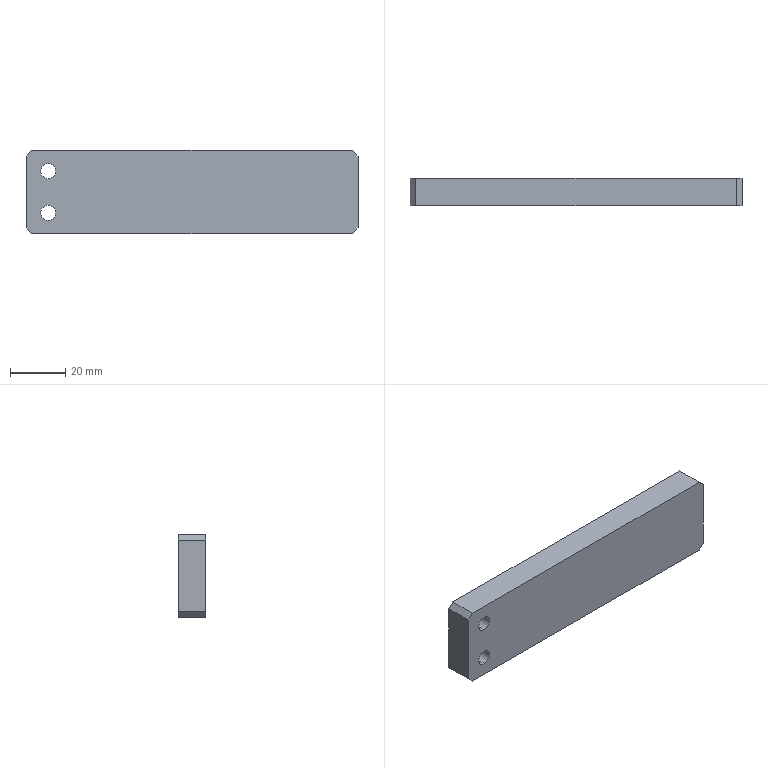Part | SolidWorks | features HoleWzd 2, BreakCorner 1, FlatPattern 1, SMBaseFlange 1, SheetMetal 1 | 1 solid | 22 faces | box 120 x 10 x 30 mm | volume 35369 mm3 | plane 10 | cylinder 8 | cone 4 | commonest cylinder face diameters 2.5 x4 5.5 x4
STEP:
#1=CARTESIAN_POINT('',(43.5,-7.5,-16.25));
#2=VERTEX_POINT('',#1);
#3=CARTESIAN_POINT('',(43.5,-7.5,-13.75));
#4=VERTEX_POINT('',#3);
#5=CARTESIAN_POINT('',(43.5,-7.5,-15.));
#6=DIRECTION('',(0.,1.,0.));
#7=DIRECTION('',(0.,0.,1.));
#8=AXIS2_PLACEMENT_3D('',#5,#6,#7);
#9=CIRCLE('',#8,1.25);
#10=EDGE_CURVE('',#2,#4,#9,.T.);
#11=ORIENTED_EDGE('',*,*,#10,.F.);
#12=CARTESIAN_POINT('',(43.5,0.,-16.25));
#13=VERTEX_POINT('',#12);
#14=CARTESIAN_POINT('',(43.5,0.,-16.25));
#15=DIRECTION('',(0.,1.,0.));
#16=VECTOR('',#15,1000.);
#17=LINE('',#14,#16);
#18=EDGE_CURVE('',#2,#13,#17,.T.);
#19=ORIENTED_EDGE('',*,*,#18,.T.);
#20=CARTESIAN_POINT('',(43.5,0.,-13.75));
#21=VERTEX_POINT('',#20);
#22=CARTESIAN_POINT('',(43.5,0.,-15.));
#23=DIRECTION('',(0.,1.,0.));
#24=DIRECTION('',(0.,0.,1.));
#25=AXIS2_PLACEMENT_3D('',#22,#23,#24);
#26=CIRCLE('',#25,1.25);
#27=EDGE_CURVE('',#13,#21,#26,.T.);
#28=ORIENTED_EDGE('',*,*,#27,.T.);
#29=CARTESIAN_POINT('',(43.5,0.,-13.75));
#30=DIRECTION('',(0.,1.,0.));
#31=VECTOR('',#30,1000.);
#32=LINE('',#29,#31);
#33=EDGE_CURVE('',#4,#21,#32,.T.);
#34=ORIENTED_EDGE('',*,*,#33,.F.);
#35=EDGE_LOOP('',(#11,#19,#28,#34));
#36=FACE_OUTER_BOUND('',#35,.T.);
#37=CARTESIAN_POINT('',(43.5,0.,-15.));
#38=DIRECTION('',(0.,1.,0.));
#39=DIRECTION('',(0.,0.,1.));
#40=AXIS2_PLACEMENT_3D('',#37,#38,#39);
#41=CYLINDRICAL_SURFACE('',#40,1.25);
#42=ADVANCED_FACE('',(#36),#41,.F.);
#43=CARTESIAN_POINT('',(43.5,-8.251,-15.));
#44=VERTEX_POINT('',#43);
#45=CARTESIAN_POINT('',(43.5,-7.5,-13.75));
#46=DIRECTION('',(0.,0.515,0.8572));
#47=VECTOR('',#46,1000.);
#48=LINE('',#45,#47);
#49=EDGE_CURVE('',#44,#4,#48,.T.);
#50=ORIENTED_EDGE('',*,*,#49,.F.);
#51=CARTESIAN_POINT('',(43.5,-7.5,-16.25));
#52=DIRECTION('',(0.,0.515,-0.8572));
#53=VECTOR('',#52,1000.);
#54=LINE('',#51,#53);
#55=EDGE_CURVE('',#44,#2,#54,.T.);
#56=ORIENTED_EDGE('',*,*,#55,.T.);
#57=ORIENTED_EDGE('',*,*,#10,.T.);
#58=EDGE_LOOP('',(#50,#56,#57));
#59=FACE_OUTER_BOUND('',#58,.T.);
#60=CARTESIAN_POINT('',(43.5,-7.5,-15.));
#61=DIRECTION('',(0.,1.,0.));
#62=DIRECTION('',(0.,0.,1.));
#63=AXIS2_PLACEMENT_3D('',#60,#61,#62);
#64=CONICAL_SURFACE('',#63,1.25,1.03);
#65=ADVANCED_FACE('',(#59),#64,.F.);
#66=CARTESIAN_POINT('',(93.5,-7.5,-16.25));
#67=VERTEX_POINT('',#66);
#68=CARTESIAN_POINT('',(93.5,-7.5,-13.75));
#69=VERTEX_POINT('',#68);
#70=CARTESIAN_POINT('',(93.5,-7.5,-15.));
#71=DIRECTION('',(0.,1.,0.));
#72=DIRECTION('',(0.,0.,1.));
#73=AXIS2_PLACEMENT_3D('',#70,#71,#72);
#74=CIRCLE('',#73,1.25);
#75=EDGE_CURVE('',#67,#69,#74,.T.);
#76=ORIENTED_EDGE('',*,*,#75,.F.);
#77=CARTESIAN_POINT('',(93.5,0.,-16.25));
#78=VERTEX_POINT('',#77);
#79=CARTESIAN_POINT('',(93.5,0.,-16.25));
#80=DIRECTION('',(0.,1.,0.));
#81=VECTOR('',#80,1000.);
#82=LINE('',#79,#81);
#83=EDGE_CURVE('',#67,#78,#82,.T.);
#84=ORIENTED_EDGE('',*,*,#83,.T.);
#85=CARTESIAN_POINT('',(93.5,0.,-13.75));
#86=VERTEX_POINT('',#85);
#87=CARTESIAN_POINT('',(93.5,0.,-15.));
#88=DIRECTION('',(0.,1.,0.));
#89=DIRECTION('',(0.,0.,1.));
#90=AXIS2_PLACEMENT_3D('',#87,#88,#89);
#91=CIRCLE('',#90,1.25);
#92=EDGE_CURVE('',#78,#86,#91,.T.);
#93=ORIENTED_EDGE('',*,*,#92,.T.);
#94=CARTESIAN_POINT('',(93.5,0.,-13.75));
#95=DIRECTION('',(0.,1.,0.));
#96=VECTOR('',#95,1000.);
#97=LINE('',#94,#96);
#98=EDGE_CURVE('',#69,#86,#97,.T.);
#99=ORIENTED_EDGE('',*,*,#98,.F.);
#100=EDGE_LOOP('',(#76,#84,#93,#99));
#101=FACE_OUTER_BOUND('',#100,.T.);
#102=CARTESIAN_POINT('',(93.5,0.,-15.));
#103=DIRECTION('',(0.,1.,0.));
#104=DIRECTION('',(0.,0.,1.));
#105=AXIS2_PLACEMENT_3D('',#102,#103,#104);
#106=CYLINDRICAL_SURFACE('',#105,1.25);
#107=ADVANCED_FACE('',(#101),#106,.F.);
#108=CARTESIAN_POINT('',(93.5,-8.251,-15.));
#109=VERTEX_POINT('',#108);
#110=CARTESIAN_POINT('',(93.5,-7.5,-13.75));
#111=DIRECTION('',(0.,0.515,0.8572));
#112=VECTOR('',#111,1000.);
#113=LINE('',#110,#112);
#114=EDGE_CURVE('',#109,#69,#113,.T.);
#115=ORIENTED_EDGE('',*,*,#114,.F.);
#116=CARTESIAN_POINT('',(93.5,-7.5,-16.25));
#117=DIRECTION('',(0.,0.515,-0.8572));
#118=VECTOR('',#117,1000.);
#119=LINE('',#116,#118);
#120=EDGE_CURVE('',#109,#67,#119,.T.);
#121=ORIENTED_EDGE('',*,*,#120,.T.);
#122=ORIENTED_EDGE('',*,*,#75,.T.);
#123=EDGE_LOOP('',(#115,#121,#122));
#124=FACE_OUTER_BOUND('',#123,.T.);
#125=CARTESIAN_POINT('',(93.5,-7.5,-15.));
#126=DIRECTION('',(0.,1.,0.));
#127=DIRECTION('',(0.,0.,1.));
#128=AXIS2_PLACEMENT_3D('',#125,#126,#127);
#129=CONICAL_SURFACE('',#128,1.25,1.03);
#130=ADVANCED_FACE('',(#124),#129,.F.);
#131=CARTESIAN_POINT('',(8.,0.,-19.75));
#132=VERTEX_POINT('',#131);
#133=CARTESIAN_POINT('',(8.,0.,-25.25));
#134=VERTEX_POINT('',#133);
#135=CARTESIAN_POINT('',(8.,0.,-22.5));
#136=DIRECTION('',(0.,-1.,0.));
#137=DIRECTION('',(0.,0.,-1.));
#138=AXIS2_PLACEMENT_3D('',#135,#136,#137);
#139=CIRCLE('',#138,2.75);
#140=EDGE_CURVE('',#132,#134,#139,.T.);
#141=ORIENTED_EDGE('',*,*,#140,.F.);
#142=CARTESIAN_POINT('',(8.,-10.,-19.75));
#143=VERTEX_POINT('',#142);
#144=CARTESIAN_POINT('',(8.,-10.,-19.75));
#145=DIRECTION('',(0.,-1.,0.));
#146=VECTOR('',#145,1000.);
#147=LINE('',#144,#146);
#148=EDGE_CURVE('',#132,#143,#147,.T.);
#149=ORIENTED_EDGE('',*,*,#148,.T.);
#150=CARTESIAN_POINT('',(8.,-10.,-25.25));
#151=VERTEX_POINT('',#150);
#152=CARTESIAN_POINT('',(8.,-10.,-22.5));
#153=DIRECTION('',(0.,-1.,0.));
#154=DIRECTION('',(0.,0.,-1.));
#155=AXIS2_PLACEMENT_3D('',#152,#153,#154);
#156=CIRCLE('',#155,2.75);
#157=EDGE_CURVE('',#143,#151,#156,.T.);
#158=ORIENTED_EDGE('',*,*,#157,.T.);
#159=CARTESIAN_POINT('',(8.,-10.,-25.25));
#160=DIRECTION('',(0.,-1.,0.));
#161=VECTOR('',#160,1000.);
#162=LINE('',#159,#161);
#163=EDGE_CURVE('',#134,#151,#162,.T.);
#164=ORIENTED_EDGE('',*,*,#163,.F.);
#165=EDGE_LOOP('',(#141,#149,#158,#164));
#166=FACE_OUTER_BOUND('',#165,.T.);
#167=CARTESIAN_POINT('',(8.,-10.,-22.5));
#168=DIRECTION('',(0.,-1.,0.));
#169=DIRECTION('',(0.,0.,-1.));
#170=AXIS2_PLACEMENT_3D('',#167,#168,#169);
#171=CYLINDRICAL_SURFACE('',#170,2.75);
#172=ADVANCED_FACE('',(#166),#171,.F.);
#173=CARTESIAN_POINT('',(8.,0.,-4.75));
#174=VERTEX_POINT('',#173);
#175=CARTESIAN_POINT('',(8.,0.,-10.25));
#176=VERTEX_POINT('',#175);
#177=CARTESIAN_POINT('',(8.,0.,-7.5));
#178=DIRECTION('',(0.,-1.,0.));
#179=DIRECTION('',(0.,0.,-1.));
#180=AXIS2_PLACEMENT_3D('',#177,#178,#179);
#181=CIRCLE('',#180,2.75);
#182=EDGE_CURVE('',#174,#176,#181,.T.);
#183=ORIENTED_EDGE('',*,*,#182,.F.);
#184=CARTESIAN_POINT('',(8.,-10.,-4.75));
#185=VERTEX_POINT('',#184);
#186=CARTESIAN_POINT('',(8.,-10.,-4.75));
#187=DIRECTION('',(0.,-1.,0.));
#188=VECTOR('',#187,1000.);
#189=LINE('',#186,#188);
#190=EDGE_CURVE('',#174,#185,#189,.T.);
#191=ORIENTED_EDGE('',*,*,#190,.T.);
#192=CARTESIAN_POINT('',(8.,-10.,-10.25));
#193=VERTEX_POINT('',#192);
#194=CARTESIAN_POINT('',(8.,-10.,-7.5));
#195=DIRECTION('',(0.,-1.,0.));
#196=DIRECTION('',(0.,0.,-1.));
#197=AXIS2_PLACEMENT_3D('',#194,#195,#196);
#198=CIRCLE('',#197,2.75);
#199=EDGE_CURVE('',#185,#193,#198,.T.);
#200=ORIENTED_EDGE('',*,*,#199,.T.);
#201=CARTESIAN_POINT('',(8.,-10.,-10.25));
#202=DIRECTION('',(0.,-1.,0.));
#203=VECTOR('',#202,1000.);
#204=LINE('',#201,#203);
#205=EDGE_CURVE('',#176,#193,#204,.T.);
#206=ORIENTED_EDGE('',*,*,#205,.F.);
#207=EDGE_LOOP('',(#183,#191,#200,#206));
#208=FACE_OUTER_BOUND('',#207,.T.);
#209=CARTESIAN_POINT('',(8.,-10.,-7.5));
#210=DIRECTION('',(0.,-1.,0.));
#211=DIRECTION('',(0.,0.,-1.));
#212=AXIS2_PLACEMENT_3D('',#209,#210,#211);
#213=CYLINDRICAL_SURFACE('',#212,2.75);
#214=ADVANCED_FACE('',(#208),#213,.F.);
#215=CARTESIAN_POINT('',(0.,-10.,-28.));
#216=VERTEX_POINT('',#215);
#217=CARTESIAN_POINT('',(0.,-10.,-2.));
#218=VERTEX_POINT('',#217);
#219=CARTESIAN_POINT('',(0.,-10.,0.));
#220=DIRECTION('',(0.,0.,1.));
#221=VECTOR('',#220,1000.);
#222=LINE('',#219,#221);
#223=EDGE_CURVE('',#216,#218,#222,.T.);
#224=ORIENTED_EDGE('',*,*,#223,.T.);
#225=CARTESIAN_POINT('',(0.,0.,-2.));
#226=VERTEX_POINT('',#225);
#227=CARTESIAN_POINT('',(0.,-10.,-2.));
#228=DIRECTION('',(0.,1.,0.));
#229=VECTOR('',#228,1000.);
#230=LINE('',#227,#229);
#231=EDGE_CURVE('',#218,#226,#230,.T.);
#232=ORIENTED_EDGE('',*,*,#231,.T.);
#233=CARTESIAN_POINT('',(0.,0.,-28.));
#234=VERTEX_POINT('',#233);
#235=CARTESIAN_POINT('',(0.,0.,0.));
#236=DIRECTION('',(0.,0.,1.));
#237=VECTOR('',#236,1000.);
#238=LINE('',#235,#237);
#239=EDGE_CURVE('',#234,#226,#238,.T.);
#240=ORIENTED_EDGE('',*,*,#239,.F.);
#241=CARTESIAN_POINT('',(0.,-10.,-28.));
#242=DIRECTION('',(0.,-1.,0.));
#243=VECTOR('',#242,1000.);
#244=LINE('',#241,#243);
#245=EDGE_CURVE('',#234,#216,#244,.T.);
#246=ORIENTED_EDGE('',*,*,#245,.T.);
#247=EDGE_LOOP('',(#224,#232,#240,#246));
#248=FACE_OUTER_BOUND('',#247,.T.);
#249=CARTESIAN_POINT('',(0.,-10.,0.));
#250=DIRECTION('',(-1.,0.,0.));
#251=DIRECTION('',(0.,0.,1.));
#252=AXIS2_PLACEMENT_3D('',#249,#250,#251);
#253=PLANE('',#252);
#254=ADVANCED_FACE('',(#248),#253,.T.);
#255=CARTESIAN_POINT('',(118.,0.,-30.));
#256=VERTEX_POINT('',#255);
#257=CARTESIAN_POINT('',(2.,0.,-30.));
#258=VERTEX_POINT('',#257);
#259=CARTESIAN_POINT('',(0.,0.,-30.));
#260=DIRECTION('',(-1.,0.,0.));
#261=VECTOR('',#260,1000.);
#262=LINE('',#259,#261);
#263=EDGE_CURVE('',#256,#258,#262,.T.);
#264=ORIENTED_EDGE('',*,*,#263,.F.);
#265=CARTESIAN_POINT('',(118.,-10.,-30.));
#266=VERTEX_POINT('',#265);
#267=CARTESIAN_POINT('',(118.,-10.,-30.));
#268=DIRECTION('',(0.,-1.,0.));
#269=VECTOR('',#268,1000.);
#270=LINE('',#267,#269);
#271=EDGE_CURVE('',#256,#266,#270,.T.);
#272=ORIENTED_EDGE('',*,*,#271,.T.);
#273=CARTESIAN_POINT('',(2.,-10.,-30.));
#274=VERTEX_POINT('',#273);
#275=CARTESIAN_POINT('',(0.,-10.,-30.));
#276=DIRECTION('',(-1.,0.,0.));
#277=VECTOR('',#276,1000.);
#278=LINE('',#275,#277);
#279=EDGE_CURVE('',#266,#274,#278,.T.);
#280=ORIENTED_EDGE('',*,*,#279,.T.);
#281=CARTESIAN_POINT('',(2.,-10.,-30.));
#282=DIRECTION('',(0.,1.,0.));
#283=VECTOR('',#282,1000.);
#284=LINE('',#281,#283);
#285=EDGE_CURVE('',#274,#258,#284,.T.);
#286=ORIENTED_EDGE('',*,*,#285,.T.);
#287=EDGE_LOOP('',(#264,#272,#280,#286));
#288=FACE_OUTER_BOUND('',#287,.T.);
#289=CARTESIAN_POINT('',(0.,-10.,-30.));
#290=DIRECTION('',(0.,0.,-1.));
#291=DIRECTION('',(-1.,0.,0.));
#292=AXIS2_PLACEMENT_3D('',#289,#290,#291);
#293=PLANE('',#292);
#294=ADVANCED_FACE('',(#288),#293,.T.);
#295=CARTESIAN_POINT('',(120.,0.,-2.));
#296=VERTEX_POINT('',#295);
#297=CARTESIAN_POINT('',(120.,0.,-28.));
#298=VERTEX_POINT('',#297);
#299=CARTESIAN_POINT('',(120.,0.,0.));
#300=DIRECTION('',(0.,0.,-1.));
#301=VECTOR('',#300,1000.);
#302=LINE('',#299,#301);
#303=EDGE_CURVE('',#296,#298,#302,.T.);
#304=ORIENTED_EDGE('',*,*,#303,.F.);
#305=CARTESIAN_POINT('',(120.,-10.,-2.));
#306=VERTEX_POINT('',#305);
#307=CARTESIAN_POINT('',(120.,-10.,-2.));
#308=DIRECTION('',(0.,-1.,0.));
#309=VECTOR('',#308,1000.);
#310=LINE('',#307,#309);
#311=EDGE_CURVE('',#296,#306,#310,.T.);
#312=ORIENTED_EDGE('',*,*,#311,.T.);
#313=CARTESIAN_POINT('',(120.,-10.,-28.));
#314=VERTEX_POINT('',#313);
#315=CARTESIAN_POINT('',(120.,-10.,0.));
#316=DIRECTION('',(0.,0.,-1.));
#317=VECTOR('',#316,1000.);
#318=LINE('',#315,#317);
#319=EDGE_CURVE('',#306,#314,#318,.T.);
#320=ORIENTED_EDGE('',*,*,#319,.T.);
#321=CARTESIAN_POINT('',(120.,-10.,-28.));
#322=DIRECTION('',(0.,1.,0.));
#323=VECTOR('',#322,1000.);
#324=LINE('',#321,#323);
#325=EDGE_CURVE('',#314,#298,#324,.T.);
#326=ORIENTED_EDGE('',*,*,#325,.T.);
#327=EDGE_LOOP('',(#304,#312,#320,#326));
#328=FACE_OUTER_BOUND('',#327,.T.);
#329=CARTESIAN_POINT('',(120.,-10.,0.));
#330=DIRECTION('',(1.,0.,0.));
#331=DIRECTION('',(0.,0.,-1.));
#332=AXIS2_PLACEMENT_3D('',#329,#330,#331);
#333=PLANE('',#332);
#334=ADVANCED_FACE('',(#328),#333,.T.);
#335=CARTESIAN_POINT('',(2.,0.,0.));
#336=VERTEX_POINT('',#335);
#337=CARTESIAN_POINT('',(118.,0.,0.));
#338=VERTEX_POINT('',#337);
#339=CARTESIAN_POINT('',(0.,0.,0.));
#340=DIRECTION('',(1.,0.,0.));
#341=VECTOR('',#340,1000.);
#342=LINE('',#339,#341);
#343=EDGE_CURVE('',#336,#338,#342,.T.);
#344=ORIENTED_EDGE('',*,*,#343,.F.);
#345=CARTESIAN_POINT('',(2.,-10.,0.));
#346=VERTEX_POINT('',#345);
#347=CARTESIAN_POINT('',(2.,-10.,0.));
#348=DIRECTION('',(0.,-1.,0.));
#349=VECTOR('',#348,1000.);
#350=LINE('',#347,#349);
#351=EDGE_CURVE('',#336,#346,#350,.T.);
#352=ORIENTED_EDGE('',*,*,#351,.T.);
#353=CARTESIAN_POINT('',(118.,-10.,0.));
#354=VERTEX_POINT('',#353);
#355=CARTESIAN_POINT('',(0.,-10.,0.));
#356=DIRECTION('',(1.,0.,0.));
#357=VECTOR('',#356,1000.);
#358=LINE('',#355,#357);
#359=EDGE_CURVE('',#346,#354,#358,.T.);
#360=ORIENTED_EDGE('',*,*,#359,.T.);
#361=CARTESIAN_POINT('',(118.,-10.,0.));
#362=DIRECTION('',(0.,1.,0.));
#363=VECTOR('',#362,1000.);
#364=LINE('',#361,#363);
#365=EDGE_CURVE('',#354,#338,#364,.T.);
#366=ORIENTED_EDGE('',*,*,#365,.T.);
#367=EDGE_LOOP('',(#344,#352,#360,#366));
#368=FACE_OUTER_BOUND('',#367,.T.);
#369=CARTESIAN_POINT('',(0.,-10.,0.));
#370=DIRECTION('',(0.,0.,1.));
#371=DIRECTION('',(1.,0.,0.));
#372=AXIS2_PLACEMENT_3D('',#369,#370,#371);
#373=PLANE('',#372);
#374=ADVANCED_FACE('',(#368),#373,.T.);
#375=CARTESIAN_POINT('',(8.,-10.,-22.5));
#376=DIRECTION('',(0.,-1.,0.));
#377=DIRECTION('',(0.,0.,-1.));
#378=AXIS2_PLACEMENT_3D('',#375,#376,#377);
#379=CIRCLE('',#378,2.75);
#380=EDGE_CURVE('',#151,#143,#379,.T.);
#381=ORIENTED_EDGE('',*,*,#380,.F.);
#382=ORIENTED_EDGE('',*,*,#157,.F.);
#383=EDGE_LOOP('',(#381,#382));
#384=FACE_BOUND('',#383,.T.);
#385=CARTESIAN_POINT('',(8.,-10.,-7.5));
#386=DIRECTION('',(0.,-1.,0.));
#387=DIRECTION('',(0.,0.,-1.));
#388=AXIS2_PLACEMENT_3D('',#385,#386,#387);
#389=CIRCLE('',#388,2.75);
#390=EDGE_CURVE('',#193,#185,#389,.T.);
#391=ORIENTED_EDGE('',*,*,#390,.F.);
#392=ORIENTED_EDGE('',*,*,#199,.F.);
#393=EDGE_LOOP('',(#391,#392));
#394=FACE_BOUND('',#393,.T.);
#395=ORIENTED_EDGE('',*,*,#359,.F.);
#396=CARTESIAN_POINT('',(1.,-10.,-1.));
#397=DIRECTION('',(-0.7071,0.,-0.7071));
#398=VECTOR('',#397,1000.);
#399=LINE('',#396,#398);
#400=EDGE_CURVE('',#346,#218,#399,.T.);
#401=ORIENTED_EDGE('',*,*,#400,.T.);
#402=ORIENTED_EDGE('',*,*,#223,.F.);
#403=CARTESIAN_POINT('',(-14.,-10.,-14.));
#404=DIRECTION('',(0.7071,0.,-0.7071));
#405=VECTOR('',#404,1000.);
#406=LINE('',#403,#405);
#407=EDGE_CURVE('',#216,#274,#406,.T.);
#408=ORIENTED_EDGE('',*,*,#407,.T.);
#409=ORIENTED_EDGE('',*,*,#279,.F.);
#410=CARTESIAN_POINT('',(74.,-10.,-74.));
#411=DIRECTION('',(0.7071,0.,0.7071));
#412=VECTOR('',#411,1000.);
#413=LINE('',#410,#412);
#414=EDGE_CURVE('',#266,#314,#413,.T.);
#415=ORIENTED_EDGE('',*,*,#414,.T.);
#416=ORIENTED_EDGE('',*,*,#319,.F.);
#417=CARTESIAN_POINT('',(59.,-10.,59.));
#418=DIRECTION('',(-0.7071,0.,0.7071));
#419=VECTOR('',#418,1000.);
#420=LINE('',#417,#419);
#421=EDGE_CURVE('',#306,#354,#420,.T.);
#422=ORIENTED_EDGE('',*,*,#421,.T.);
#423=EDGE_LOOP('',(#395,#401,#402,#408,#409,#415,#416,#422));
#424=FACE_OUTER_BOUND('',#423,.T.);
#425=CARTESIAN_POINT('',(0.,-10.,0.));
#426=DIRECTION('',(0.,-1.,0.));
#427=DIRECTION('',(0.,0.,-1.));
#428=AXIS2_PLACEMENT_3D('',#425,#426,#427);
#429=PLANE('',#428);
#430=ADVANCED_FACE('',(#384,#394,#424),#429,.T.);
#431=CARTESIAN_POINT('',(43.5,0.,-15.));
#432=DIRECTION('',(0.,1.,0.));
#433=DIRECTION('',(0.,0.,1.));
#434=AXIS2_PLACEMENT_3D('',#431,#432,#433);
#435=CIRCLE('',#434,1.25);
#436=EDGE_CURVE('',#21,#13,#435,.T.);
#437=ORIENTED_EDGE('',*,*,#436,.F.);
#438=ORIENTED_EDGE('',*,*,#27,.F.);
#439=EDGE_LOOP('',(#437,#438));
#440=FACE_BOUND('',#439,.T.);
#441=CARTESIAN_POINT('',(93.5,0.,-15.));
#442=DIRECTION('',(0.,1.,0.));
#443=DIRECTION('',(0.,0.,1.));
#444=AXIS2_PLACEMENT_3D('',#441,#442,#443);
#445=CIRCLE('',#444,1.25);
#446=EDGE_CURVE('',#86,#78,#445,.T.);
#447=ORIENTED_EDGE('',*,*,#446,.F.);
#448=ORIENTED_EDGE('',*,*,#92,.F.);
#449=EDGE_LOOP('',(#447,#448));
#450=FACE_BOUND('',#449,.T.);
#451=CARTESIAN_POINT('',(8.,0.,-22.5));
#452=DIRECTION('',(0.,-1.,0.));
#453=DIRECTION('',(0.,0.,-1.));
#454=AXIS2_PLACEMENT_3D('',#451,#452,#453);
#455=CIRCLE('',#454,2.75);
#456=EDGE_CURVE('',#134,#132,#455,.T.);
#457=ORIENTED_EDGE('',*,*,#456,.T.);
#458=ORIENTED_EDGE('',*,*,#140,.T.);
#459=EDGE_LOOP('',(#457,#458));
#460=FACE_BOUND('',#459,.T.);
#461=CARTESIAN_POINT('',(8.,0.,-7.5));
#462=DIRECTION('',(0.,-1.,0.));
#463=DIRECTION('',(0.,0.,-1.));
#464=AXIS2_PLACEMENT_3D('',#461,#462,#463);
#465=CIRCLE('',#464,2.75);
#466=EDGE_CURVE('',#176,#174,#465,.T.);
#467=ORIENTED_EDGE('',*,*,#466,.T.);
#468=ORIENTED_EDGE('',*,*,#182,.T.);
#469=EDGE_LOOP('',(#467,#468));
#470=FACE_BOUND('',#469,.T.);
#471=ORIENTED_EDGE('',*,*,#239,.T.);
#472=CARTESIAN_POINT('',(0.,0.,-2.));
#473=DIRECTION('',(0.7071,0.,0.7071));
#474=VECTOR('',#473,1000.);
#475=LINE('',#472,#474);
#476=EDGE_CURVE('',#226,#336,#475,.T.);
#477=ORIENTED_EDGE('',*,*,#476,.T.);
#478=ORIENTED_EDGE('',*,*,#343,.T.);
#479=CARTESIAN_POINT('',(118.,0.,0.));
#480=DIRECTION('',(0.7071,0.,-0.7071));
#481=VECTOR('',#480,1000.);
#482=LINE('',#479,#481);
#483=EDGE_CURVE('',#338,#296,#482,.T.);
#484=ORIENTED_EDGE('',*,*,#483,.T.);
#485=ORIENTED_EDGE('',*,*,#303,.T.);
#486=CARTESIAN_POINT('',(120.,0.,-28.));
#487=DIRECTION('',(-0.7071,0.,-0.7071));
#488=VECTOR('',#487,1000.);
#489=LINE('',#486,#488);
#490=EDGE_CURVE('',#298,#256,#489,.T.);
#491=ORIENTED_EDGE('',*,*,#490,.T.);
#492=ORIENTED_EDGE('',*,*,#263,.T.);
#493=CARTESIAN_POINT('',(2.,0.,-30.));
#494=DIRECTION('',(-0.7071,0.,0.7071));
#495=VECTOR('',#494,1000.);
#496=LINE('',#493,#495);
#497=EDGE_CURVE('',#258,#234,#496,.T.);
#498=ORIENTED_EDGE('',*,*,#497,.T.);
#499=EDGE_LOOP('',(#471,#477,#478,#484,#485,#491,#492,#498));
#500=FACE_OUTER_BOUND('',#499,.T.);
#501=CARTESIAN_POINT('',(0.,0.,0.));
#502=DIRECTION('',(0.,-1.,0.));
#503=DIRECTION('',(0.,0.,-1.));
#504=AXIS2_PLACEMENT_3D('',#501,#502,#503);
#505=PLANE('',#504);
#506=ADVANCED_FACE('',(#440,#450,#460,#470,#500),#505,.F.);
#507=ORIENTED_EDGE('',*,*,#407,.F.);
#508=ORIENTED_EDGE('',*,*,#245,.F.);
#509=ORIENTED_EDGE('',*,*,#497,.F.);
#510=ORIENTED_EDGE('',*,*,#285,.F.);
#511=EDGE_LOOP('',(#507,#508,#509,#510));
#512=FACE_OUTER_BOUND('',#511,.T.);
#513=CARTESIAN_POINT('',(2.,-10.,-30.));
#514=DIRECTION('',(0.7071,0.,0.7071));
#515=DIRECTION('',(0.,1.,0.));
#516=AXIS2_PLACEMENT_3D('',#513,#514,#515);
#517=PLANE('',#516);
#518=ADVANCED_FACE('',(#512),#517,.F.);
#519=ORIENTED_EDGE('',*,*,#414,.F.);
#520=ORIENTED_EDGE('',*,*,#271,.F.);
#521=ORIENTED_EDGE('',*,*,#490,.F.);
#522=ORIENTED_EDGE('',*,*,#325,.F.);
#523=EDGE_LOOP('',(#519,#520,#521,#522));
#524=FACE_OUTER_BOUND('',#523,.T.);
#525=CARTESIAN_POINT('',(120.,-10.,-28.));
#526=DIRECTION('',(-0.7071,0.,0.7071));
#527=DIRECTION('',(0.,1.,0.));
#528=AXIS2_PLACEMENT_3D('',#525,#526,#527);
#529=PLANE('',#528);
#530=ADVANCED_FACE('',(#524),#529,.F.);
#531=ORIENTED_EDGE('',*,*,#421,.F.);
#532=ORIENTED_EDGE('',*,*,#311,.F.);
#533=ORIENTED_EDGE('',*,*,#483,.F.);
#534=ORIENTED_EDGE('',*,*,#365,.F.);
#535=EDGE_LOOP('',(#531,#532,#533,#534));
#536=FACE_OUTER_BOUND('',#535,.T.);
#537=CARTESIAN_POINT('',(118.,-10.,0.));
#538=DIRECTION('',(-0.7071,0.,-0.7071));
#539=DIRECTION('',(0.,1.,0.));
#540=AXIS2_PLACEMENT_3D('',#537,#538,#539);
#541=PLANE('',#540);
#542=ADVANCED_FACE('',(#536),#541,.F.);
#543=ORIENTED_EDGE('',*,*,#400,.F.);
#544=ORIENTED_EDGE('',*,*,#351,.F.);
#545=ORIENTED_EDGE('',*,*,#476,.F.);
#546=ORIENTED_EDGE('',*,*,#231,.F.);
#547=EDGE_LOOP('',(#543,#544,#545,#546));
#548=FACE_OUTER_BOUND('',#547,.T.);
#549=CARTESIAN_POINT('',(0.,-10.,-2.));
#550=DIRECTION('',(0.7071,0.,-0.7071));
#551=DIRECTION('',(0.,1.,0.));
#552=AXIS2_PLACEMENT_3D('',#549,#550,#551);
#553=PLANE('',#552);
#554=ADVANCED_FACE('',(#548),#553,.F.);
#555=ORIENTED_EDGE('',*,*,#190,.F.);
#556=ORIENTED_EDGE('',*,*,#466,.F.);
#557=ORIENTED_EDGE('',*,*,#205,.T.);
#558=ORIENTED_EDGE('',*,*,#390,.T.);
#559=EDGE_LOOP('',(#555,#556,#557,#558));
#560=FACE_OUTER_BOUND('',#559,.T.);
#561=CARTESIAN_POINT('',(8.,-10.,-7.5));
#562=DIRECTION('',(0.,-1.,0.));
#563=DIRECTION('',(0.,0.,-1.));
#564=AXIS2_PLACEMENT_3D('',#561,#562,#563);
#565=CYLINDRICAL_SURFACE('',#564,2.75);
#566=ADVANCED_FACE('',(#560),#565,.F.);
#567=ORIENTED_EDGE('',*,*,#148,.F.);
#568=ORIENTED_EDGE('',*,*,#456,.F.);
#569=ORIENTED_EDGE('',*,*,#163,.T.);
#570=ORIENTED_EDGE('',*,*,#380,.T.);
#571=EDGE_LOOP('',(#567,#568,#569,#570));
#572=FACE_OUTER_BOUND('',#571,.T.);
#573=CARTESIAN_POINT('',(8.,-10.,-22.5));
#574=DIRECTION('',(0.,-1.,0.));
#575=DIRECTION('',(0.,0.,-1.));
#576=AXIS2_PLACEMENT_3D('',#573,#574,#575);
#577=CYLINDRICAL_SURFACE('',#576,2.75);
#578=ADVANCED_FACE('',(#572),#577,.F.);
#579=ORIENTED_EDGE('',*,*,#120,.F.);
#580=ORIENTED_EDGE('',*,*,#114,.T.);
#581=CARTESIAN_POINT('',(93.5,-7.5,-15.));
#582=DIRECTION('',(0.,1.,0.));
#583=DIRECTION('',(0.,0.,1.));
#584=AXIS2_PLACEMENT_3D('',#581,#582,#583);
#585=CIRCLE('',#584,1.25);
#586=EDGE_CURVE('',#69,#67,#585,.T.);
#587=ORIENTED_EDGE('',*,*,#586,.T.);
#588=EDGE_LOOP('',(#579,#580,#587));
#589=FACE_OUTER_BOUND('',#588,.T.);
#590=CARTESIAN_POINT('',(93.5,-7.5,-15.));
#591=DIRECTION('',(0.,1.,0.));
#592=DIRECTION('',(0.,0.,1.));
#593=AXIS2_PLACEMENT_3D('',#590,#591,#592);
#594=CONICAL_SURFACE('',#593,1.25,1.03);
#595=ADVANCED_FACE('',(#589),#594,.F.);
#596=ORIENTED_EDGE('',*,*,#83,.F.);
#597=ORIENTED_EDGE('',*,*,#586,.F.);
#598=ORIENTED_EDGE('',*,*,#98,.T.);
#599=ORIENTED_EDGE('',*,*,#446,.T.);
#600=EDGE_LOOP('',(#596,#597,#598,#599));
#601=FACE_OUTER_BOUND('',#600,.T.);
#602=CARTESIAN_POINT('',(93.5,0.,-15.));
#603=DIRECTION('',(0.,1.,0.));
#604=DIRECTION('',(0.,0.,1.));
#605=AXIS2_PLACEMENT_3D('',#602,#603,#604);
#606=CYLINDRICAL_SURFACE('',#605,1.25);
#607=ADVANCED_FACE('',(#601),#606,.F.);
#608=ORIENTED_EDGE('',*,*,#55,.F.);
#609=ORIENTED_EDGE('',*,*,#49,.T.);
#610=CARTESIAN_POINT('',(43.5,-7.5,-15.));
#611=DIRECTION('',(0.,1.,0.));
#612=DIRECTION('',(0.,0.,1.));
#613=AXIS2_PLACEMENT_3D('',#610,#611,#612);
#614=CIRCLE('',#613,1.25);
#615=EDGE_CURVE('',#4,#2,#614,.T.);
#616=ORIENTED_EDGE('',*,*,#615,.T.);
#617=EDGE_LOOP('',(#608,#609,#616));
#618=FACE_OUTER_BOUND('',#617,.T.);
#619=CARTESIAN_POINT('',(43.5,-7.5,-15.));
#620=DIRECTION('',(0.,1.,0.));
#621=DIRECTION('',(0.,0.,1.));
#622=AXIS2_PLACEMENT_3D('',#619,#620,#621);
#623=CONICAL_SURFACE('',#622,1.25,1.03);
#624=ADVANCED_FACE('',(#618),#623,.F.);
#625=ORIENTED_EDGE('',*,*,#18,.F.);
#626=ORIENTED_EDGE('',*,*,#615,.F.);
#627=ORIENTED_EDGE('',*,*,#33,.T.);
#628=ORIENTED_EDGE('',*,*,#436,.T.);
#629=EDGE_LOOP('',(#625,#626,#627,#628));
#630=FACE_OUTER_BOUND('',#629,.T.);
#631=CARTESIAN_POINT('',(43.5,0.,-15.));
#632=DIRECTION('',(0.,1.,0.));
#633=DIRECTION('',(0.,0.,1.));
#634=AXIS2_PLACEMENT_3D('',#631,#632,#633);
#635=CYLINDRICAL_SURFACE('',#634,1.25);
#636=ADVANCED_FACE('',(#630),#635,.F.);
#637=CLOSED_SHELL('',(#42,#65,#107,#130,#172,#214,#254,#294,#334,#374,#430,#506,#518,#530,#542,#554,#566,#578,#595,#607,#624,#636));
#638=MANIFOLD_SOLID_BREP('',#637);
#639=CARTESIAN_POINT('',(0.,0.,0.));
#640=DIRECTION('',(0.,0.,1.));
#641=DIRECTION('',(1.,0.,0.));
#642=AXIS2_PLACEMENT_3D('',#639,#640,#641);
#643=(LENGTH_UNIT()NAMED_UNIT(*)SI_UNIT(.MILLI.,.METRE.));
#644=UNCERTAINTY_MEASURE_WITH_UNIT(LENGTH_MEASURE(0.00001),#643,'','');
#645=(NAMED_UNIT(*)PLANE_ANGLE_UNIT()SI_UNIT($,.RADIAN.));
#646=(NAMED_UNIT(*)SI_UNIT($,.STERADIAN.)SOLID_ANGLE_UNIT());
#647=(GEOMETRIC_REPRESENTATION_CONTEXT(3)GLOBAL_UNCERTAINTY_ASSIGNED_CONTEXT((#644))GLOBAL_UNIT_ASSIGNED_CONTEXT((#643,#645,#646))REPRESENTATION_CONTEXT('',''));
#648=ADVANCED_BREP_SHAPE_REPRESENTATION('',(#638,#642),#647);